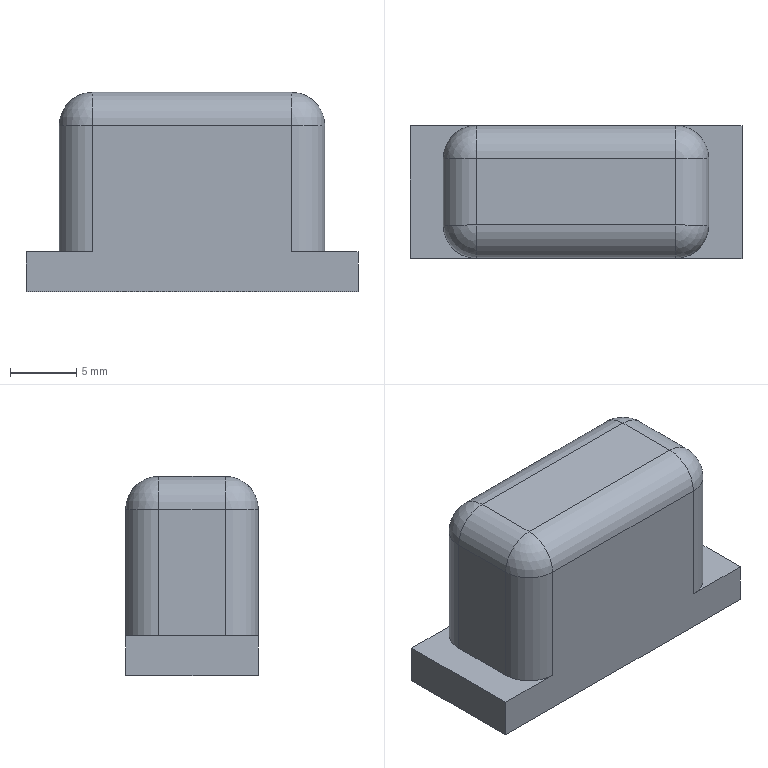Part | NX | 1 solid | 22 faces | box 25 x 10 x 15 mm | volume 3016 mm3 | plane 10 | cylinder 8 | sphere 4 | commonest cylinder face diameters 5 x8
STEP:
#1=CARTESIAN_POINT('',(151.228,185.01,0.));
#2=VERTEX_POINT('',#1);
#3=CARTESIAN_POINT('',(148.728,187.51,0.));
#4=VERTEX_POINT('',#3);
#5=CARTESIAN_POINT('',(148.728,185.01,0.));
#6=DIRECTION('',(0.,0.,1.));
#7=DIRECTION('',(1.,0.,0.));
#8=AXIS2_PLACEMENT_3D('',#5,#6,#7);
#9=CIRCLE('',#8,2.5);
#10=EDGE_CURVE('',#2,#4,#9,.T.);
#11=ORIENTED_EDGE('',*,*,#10,.F.);
#12=CARTESIAN_POINT('',(151.228,180.01,0.));
#13=VERTEX_POINT('',#12);
#14=CARTESIAN_POINT('',(151.228,180.01,0.));
#15=DIRECTION('',(0.,1.,0.));
#16=VECTOR('',#15,1000.);
#17=LINE('',#14,#16);
#18=EDGE_CURVE('',#13,#2,#17,.T.);
#19=ORIENTED_EDGE('',*,*,#18,.F.);
#20=CARTESIAN_POINT('',(148.728,177.51,0.));
#21=VERTEX_POINT('',#20);
#22=CARTESIAN_POINT('',(148.728,180.01,0.));
#23=DIRECTION('',(0.,0.,1.));
#24=DIRECTION('',(1.,0.,0.));
#25=AXIS2_PLACEMENT_3D('',#22,#23,#24);
#26=CIRCLE('',#25,2.5);
#27=EDGE_CURVE('',#21,#13,#26,.T.);
#28=ORIENTED_EDGE('',*,*,#27,.F.);
#29=CARTESIAN_POINT('',(153.728,177.51,0.));
#30=VERTEX_POINT('',#29);
#31=CARTESIAN_POINT('',(153.728,177.51,0.));
#32=DIRECTION('',(-1.,0.,0.));
#33=VECTOR('',#32,1000.);
#34=LINE('',#31,#33);
#35=EDGE_CURVE('',#30,#21,#34,.T.);
#36=ORIENTED_EDGE('',*,*,#35,.F.);
#37=CARTESIAN_POINT('',(153.728,187.51,0.));
#38=VERTEX_POINT('',#37);
#39=CARTESIAN_POINT('',(153.728,187.51,0.));
#40=DIRECTION('',(0.,-1.,0.));
#41=VECTOR('',#40,1000.);
#42=LINE('',#39,#41);
#43=EDGE_CURVE('',#38,#30,#42,.T.);
#44=ORIENTED_EDGE('',*,*,#43,.F.);
#45=CARTESIAN_POINT('',(128.728,187.51,0.));
#46=DIRECTION('',(1.,0.,0.));
#47=VECTOR('',#46,1000.);
#48=LINE('',#45,#47);
#49=EDGE_CURVE('',#4,#38,#48,.T.);
#50=ORIENTED_EDGE('',*,*,#49,.F.);
#51=EDGE_LOOP('',(#11,#19,#28,#36,#44,#50));
#52=FACE_BOUND('',#51,.T.);
#53=CARTESIAN_POINT('',(0.,0.,0.));
#54=DIRECTION('',(0.,0.,-1.));
#55=DIRECTION('',(-1.,0.,0.));
#56=AXIS2_PLACEMENT_3D('',#53,#54,#55);
#57=PLANE('',#56);
#58=ADVANCED_FACE('',(#52),#57,.F.);
#59=CARTESIAN_POINT('',(133.728,187.51,0.));
#60=VERTEX_POINT('',#59);
#61=CARTESIAN_POINT('',(131.228,185.01,0.));
#62=VERTEX_POINT('',#61);
#63=CARTESIAN_POINT('',(133.728,185.01,0.));
#64=DIRECTION('',(0.,0.,1.));
#65=DIRECTION('',(1.,0.,0.));
#66=AXIS2_PLACEMENT_3D('',#63,#64,#65);
#67=CIRCLE('',#66,2.5);
#68=EDGE_CURVE('',#60,#62,#67,.T.);
#69=ORIENTED_EDGE('',*,*,#68,.F.);
#70=CARTESIAN_POINT('',(128.728,187.51,0.));
#71=VERTEX_POINT('',#70);
#72=CARTESIAN_POINT('',(128.728,187.51,0.));
#73=DIRECTION('',(1.,0.,0.));
#74=VECTOR('',#73,1000.);
#75=LINE('',#72,#74);
#76=EDGE_CURVE('',#71,#60,#75,.T.);
#77=ORIENTED_EDGE('',*,*,#76,.F.);
#78=CARTESIAN_POINT('',(128.728,177.51,0.));
#79=VERTEX_POINT('',#78);
#80=CARTESIAN_POINT('',(128.728,177.51,0.));
#81=DIRECTION('',(0.,1.,0.));
#82=VECTOR('',#81,1000.);
#83=LINE('',#80,#82);
#84=EDGE_CURVE('',#79,#71,#83,.T.);
#85=ORIENTED_EDGE('',*,*,#84,.F.);
#86=CARTESIAN_POINT('',(133.728,177.51,0.));
#87=VERTEX_POINT('',#86);
#88=CARTESIAN_POINT('',(153.728,177.51,0.));
#89=DIRECTION('',(-1.,0.,0.));
#90=VECTOR('',#89,1000.);
#91=LINE('',#88,#90);
#92=EDGE_CURVE('',#87,#79,#91,.T.);
#93=ORIENTED_EDGE('',*,*,#92,.F.);
#94=CARTESIAN_POINT('',(131.228,180.01,0.));
#95=VERTEX_POINT('',#94);
#96=CARTESIAN_POINT('',(133.728,180.01,0.));
#97=DIRECTION('',(0.,0.,1.));
#98=DIRECTION('',(1.,0.,0.));
#99=AXIS2_PLACEMENT_3D('',#96,#97,#98);
#100=CIRCLE('',#99,2.5);
#101=EDGE_CURVE('',#95,#87,#100,.T.);
#102=ORIENTED_EDGE('',*,*,#101,.F.);
#103=CARTESIAN_POINT('',(131.228,185.01,0.));
#104=DIRECTION('',(0.,-1.,0.));
#105=VECTOR('',#104,1000.);
#106=LINE('',#103,#105);
#107=EDGE_CURVE('',#62,#95,#106,.T.);
#108=ORIENTED_EDGE('',*,*,#107,.F.);
#109=EDGE_LOOP('',(#69,#77,#85,#93,#102,#108));
#110=FACE_BOUND('',#109,.T.);
#111=CARTESIAN_POINT('',(0.,0.,0.));
#112=DIRECTION('',(0.,0.,-1.));
#113=DIRECTION('',(-1.,0.,0.));
#114=AXIS2_PLACEMENT_3D('',#111,#112,#113);
#115=PLANE('',#114);
#116=ADVANCED_FACE('',(#110),#115,.F.);
#117=CARTESIAN_POINT('',(148.728,177.51,9.5));
#118=VERTEX_POINT('',#117);
#119=CARTESIAN_POINT('',(148.728,177.51,0.));
#120=DIRECTION('',(0.,0.,1.));
#121=VECTOR('',#120,1000.);
#122=LINE('',#119,#121);
#123=EDGE_CURVE('',#21,#118,#122,.T.);
#124=ORIENTED_EDGE('',*,*,#123,.T.);
#125=CARTESIAN_POINT('',(133.728,177.51,9.5));
#126=VERTEX_POINT('',#125);
#127=CARTESIAN_POINT('',(153.728,177.51,9.5));
#128=DIRECTION('',(1.,0.,0.));
#129=VECTOR('',#128,1000.);
#130=LINE('',#127,#129);
#131=EDGE_CURVE('',#118,#126,#130,.F.);
#132=ORIENTED_EDGE('',*,*,#131,.T.);
#133=CARTESIAN_POINT('',(133.728,177.51,0.));
#134=DIRECTION('',(0.,0.,1.));
#135=VECTOR('',#134,1000.);
#136=LINE('',#133,#135);
#137=EDGE_CURVE('',#87,#126,#136,.T.);
#138=ORIENTED_EDGE('',*,*,#137,.F.);
#139=ORIENTED_EDGE('',*,*,#92,.T.);
#140=CARTESIAN_POINT('',(128.728,177.51,-3.));
#141=VERTEX_POINT('',#140);
#142=CARTESIAN_POINT('',(128.728,177.51,0.));
#143=DIRECTION('',(0.,0.,-1.));
#144=VECTOR('',#143,1000.);
#145=LINE('',#142,#144);
#146=EDGE_CURVE('',#79,#141,#145,.T.);
#147=ORIENTED_EDGE('',*,*,#146,.T.);
#148=CARTESIAN_POINT('',(153.728,177.51,-3.));
#149=VERTEX_POINT('',#148);
#150=CARTESIAN_POINT('',(153.728,177.51,-3.));
#151=DIRECTION('',(-1.,0.,0.));
#152=VECTOR('',#151,1000.);
#153=LINE('',#150,#152);
#154=EDGE_CURVE('',#149,#141,#153,.T.);
#155=ORIENTED_EDGE('',*,*,#154,.F.);
#156=CARTESIAN_POINT('',(153.728,177.51,0.));
#157=DIRECTION('',(0.,0.,-1.));
#158=VECTOR('',#157,1000.);
#159=LINE('',#156,#158);
#160=EDGE_CURVE('',#30,#149,#159,.T.);
#161=ORIENTED_EDGE('',*,*,#160,.F.);
#162=ORIENTED_EDGE('',*,*,#35,.T.);
#163=EDGE_LOOP('',(#124,#132,#138,#139,#147,#155,#161,#162));
#164=FACE_BOUND('',#163,.T.);
#165=CARTESIAN_POINT('',(153.728,177.51,0.));
#166=DIRECTION('',(0.,-1.,0.));
#167=DIRECTION('',(0.,0.,-1.));
#168=AXIS2_PLACEMENT_3D('',#165,#166,#167);
#169=PLANE('',#168);
#170=ADVANCED_FACE('',(#164),#169,.T.);
#171=CARTESIAN_POINT('',(128.728,187.51,-3.));
#172=VERTEX_POINT('',#171);
#173=CARTESIAN_POINT('',(128.728,177.51,-3.));
#174=DIRECTION('',(0.,1.,0.));
#175=VECTOR('',#174,1000.);
#176=LINE('',#173,#175);
#177=EDGE_CURVE('',#141,#172,#176,.T.);
#178=ORIENTED_EDGE('',*,*,#177,.F.);
#179=ORIENTED_EDGE('',*,*,#146,.F.);
#180=ORIENTED_EDGE('',*,*,#84,.T.);
#181=CARTESIAN_POINT('',(128.728,187.51,0.));
#182=DIRECTION('',(0.,0.,-1.));
#183=VECTOR('',#182,1000.);
#184=LINE('',#181,#183);
#185=EDGE_CURVE('',#71,#172,#184,.T.);
#186=ORIENTED_EDGE('',*,*,#185,.T.);
#187=EDGE_LOOP('',(#178,#179,#180,#186));
#188=FACE_BOUND('',#187,.T.);
#189=CARTESIAN_POINT('',(128.728,177.51,0.));
#190=DIRECTION('',(-1.,0.,0.));
#191=DIRECTION('',(0.,0.,1.));
#192=AXIS2_PLACEMENT_3D('',#189,#190,#191);
#193=PLANE('',#192);
#194=ADVANCED_FACE('',(#188),#193,.T.);
#195=CARTESIAN_POINT('',(133.728,187.51,9.5));
#196=VERTEX_POINT('',#195);
#197=CARTESIAN_POINT('',(133.728,187.51,0.));
#198=DIRECTION('',(0.,0.,1.));
#199=VECTOR('',#198,1000.);
#200=LINE('',#197,#199);
#201=EDGE_CURVE('',#60,#196,#200,.T.);
#202=ORIENTED_EDGE('',*,*,#201,.T.);
#203=CARTESIAN_POINT('',(148.728,187.51,9.5));
#204=VERTEX_POINT('',#203);
#205=CARTESIAN_POINT('',(128.728,187.51,9.5));
#206=DIRECTION('',(-1.,0.,0.));
#207=VECTOR('',#206,1000.);
#208=LINE('',#205,#207);
#209=EDGE_CURVE('',#196,#204,#208,.F.);
#210=ORIENTED_EDGE('',*,*,#209,.T.);
#211=CARTESIAN_POINT('',(148.728,187.51,0.));
#212=DIRECTION('',(0.,0.,1.));
#213=VECTOR('',#212,1000.);
#214=LINE('',#211,#213);
#215=EDGE_CURVE('',#4,#204,#214,.T.);
#216=ORIENTED_EDGE('',*,*,#215,.F.);
#217=ORIENTED_EDGE('',*,*,#49,.T.);
#218=CARTESIAN_POINT('',(153.728,187.51,-3.));
#219=VERTEX_POINT('',#218);
#220=CARTESIAN_POINT('',(153.728,187.51,0.));
#221=DIRECTION('',(0.,0.,-1.));
#222=VECTOR('',#221,1000.);
#223=LINE('',#220,#222);
#224=EDGE_CURVE('',#38,#219,#223,.T.);
#225=ORIENTED_EDGE('',*,*,#224,.T.);
#226=CARTESIAN_POINT('',(128.728,187.51,-3.));
#227=DIRECTION('',(1.,0.,0.));
#228=VECTOR('',#227,1000.);
#229=LINE('',#226,#228);
#230=EDGE_CURVE('',#172,#219,#229,.T.);
#231=ORIENTED_EDGE('',*,*,#230,.F.);
#232=ORIENTED_EDGE('',*,*,#185,.F.);
#233=ORIENTED_EDGE('',*,*,#76,.T.);
#234=EDGE_LOOP('',(#202,#210,#216,#217,#225,#231,#232,#233));
#235=FACE_BOUND('',#234,.T.);
#236=CARTESIAN_POINT('',(128.728,187.51,0.));
#237=DIRECTION('',(0.,1.,0.));
#238=DIRECTION('',(0.,0.,1.));
#239=AXIS2_PLACEMENT_3D('',#236,#237,#238);
#240=PLANE('',#239);
#241=ADVANCED_FACE('',(#235),#240,.T.);
#242=CARTESIAN_POINT('',(153.728,187.51,-3.));
#243=DIRECTION('',(0.,-1.,0.));
#244=VECTOR('',#243,1000.);
#245=LINE('',#242,#244);
#246=EDGE_CURVE('',#219,#149,#245,.T.);
#247=ORIENTED_EDGE('',*,*,#246,.F.);
#248=ORIENTED_EDGE('',*,*,#224,.F.);
#249=ORIENTED_EDGE('',*,*,#43,.T.);
#250=ORIENTED_EDGE('',*,*,#160,.T.);
#251=EDGE_LOOP('',(#247,#248,#249,#250));
#252=FACE_BOUND('',#251,.T.);
#253=CARTESIAN_POINT('',(153.728,187.51,0.));
#254=DIRECTION('',(1.,0.,0.));
#255=DIRECTION('',(0.,0.,-1.));
#256=AXIS2_PLACEMENT_3D('',#253,#254,#255);
#257=PLANE('',#256);
#258=ADVANCED_FACE('',(#252),#257,.T.);
#259=ORIENTED_EDGE('',*,*,#154,.T.);
#260=ORIENTED_EDGE('',*,*,#177,.T.);
#261=ORIENTED_EDGE('',*,*,#230,.T.);
#262=ORIENTED_EDGE('',*,*,#246,.T.);
#263=EDGE_LOOP('',(#259,#260,#261,#262));
#264=FACE_BOUND('',#263,.T.);
#265=CARTESIAN_POINT('',(0.,0.,-3.));
#266=DIRECTION('',(0.,0.,-1.));
#267=DIRECTION('',(-1.,0.,0.));
#268=AXIS2_PLACEMENT_3D('',#265,#266,#267);
#269=PLANE('',#268);
#270=ADVANCED_FACE('',(#264),#269,.T.);
#271=CARTESIAN_POINT('',(131.228,185.01,9.5));
#272=VERTEX_POINT('',#271);
#273=CARTESIAN_POINT('',(131.228,185.01,0.));
#274=DIRECTION('',(0.,0.,1.));
#275=VECTOR('',#274,1000.);
#276=LINE('',#273,#275);
#277=EDGE_CURVE('',#62,#272,#276,.T.);
#278=ORIENTED_EDGE('',*,*,#277,.T.);
#279=CARTESIAN_POINT('',(133.728,185.01,9.5));
#280=DIRECTION('',(0.,0.,1.));
#281=DIRECTION('',(1.,0.,0.));
#282=AXIS2_PLACEMENT_3D('',#279,#280,#281);
#283=CIRCLE('',#282,2.5);
#284=EDGE_CURVE('',#272,#196,#283,.F.);
#285=ORIENTED_EDGE('',*,*,#284,.T.);
#286=ORIENTED_EDGE('',*,*,#201,.F.);
#287=ORIENTED_EDGE('',*,*,#68,.T.);
#288=EDGE_LOOP('',(#278,#285,#286,#287));
#289=FACE_BOUND('',#288,.T.);
#290=CARTESIAN_POINT('',(133.728,185.01,0.));
#291=DIRECTION('',(0.,0.,1.));
#292=DIRECTION('',(1.,0.,0.));
#293=AXIS2_PLACEMENT_3D('',#290,#291,#292);
#294=CYLINDRICAL_SURFACE('',#293,2.5);
#295=ADVANCED_FACE('',(#289),#294,.T.);
#296=CARTESIAN_POINT('',(131.228,180.01,9.5));
#297=VERTEX_POINT('',#296);
#298=CARTESIAN_POINT('',(131.228,180.01,0.));
#299=DIRECTION('',(0.,0.,1.));
#300=VECTOR('',#299,1000.);
#301=LINE('',#298,#300);
#302=EDGE_CURVE('',#95,#297,#301,.T.);
#303=ORIENTED_EDGE('',*,*,#302,.T.);
#304=CARTESIAN_POINT('',(131.228,185.01,9.5));
#305=DIRECTION('',(0.,-1.,0.));
#306=VECTOR('',#305,1000.);
#307=LINE('',#304,#306);
#308=EDGE_CURVE('',#297,#272,#307,.F.);
#309=ORIENTED_EDGE('',*,*,#308,.T.);
#310=ORIENTED_EDGE('',*,*,#277,.F.);
#311=ORIENTED_EDGE('',*,*,#107,.T.);
#312=EDGE_LOOP('',(#303,#309,#310,#311));
#313=FACE_BOUND('',#312,.T.);
#314=CARTESIAN_POINT('',(131.228,185.01,0.));
#315=DIRECTION('',(-1.,0.,0.));
#316=DIRECTION('',(0.,0.,1.));
#317=AXIS2_PLACEMENT_3D('',#314,#315,#316);
#318=PLANE('',#317);
#319=ADVANCED_FACE('',(#313),#318,.T.);
#320=ORIENTED_EDGE('',*,*,#137,.T.);
#321=CARTESIAN_POINT('',(133.728,180.01,9.5));
#322=DIRECTION('',(0.,0.,1.));
#323=DIRECTION('',(1.,0.,0.));
#324=AXIS2_PLACEMENT_3D('',#321,#322,#323);
#325=CIRCLE('',#324,2.5);
#326=EDGE_CURVE('',#126,#297,#325,.F.);
#327=ORIENTED_EDGE('',*,*,#326,.T.);
#328=ORIENTED_EDGE('',*,*,#302,.F.);
#329=ORIENTED_EDGE('',*,*,#101,.T.);
#330=EDGE_LOOP('',(#320,#327,#328,#329));
#331=FACE_BOUND('',#330,.T.);
#332=CARTESIAN_POINT('',(133.728,180.01,0.));
#333=DIRECTION('',(0.,0.,1.));
#334=DIRECTION('',(1.,0.,0.));
#335=AXIS2_PLACEMENT_3D('',#332,#333,#334);
#336=CYLINDRICAL_SURFACE('',#335,2.5);
#337=ADVANCED_FACE('',(#331),#336,.T.);
#338=CARTESIAN_POINT('',(151.228,180.01,9.5));
#339=VERTEX_POINT('',#338);
#340=CARTESIAN_POINT('',(151.228,180.01,0.));
#341=DIRECTION('',(0.,0.,1.));
#342=VECTOR('',#341,1000.);
#343=LINE('',#340,#342);
#344=EDGE_CURVE('',#13,#339,#343,.T.);
#345=ORIENTED_EDGE('',*,*,#344,.T.);
#346=CARTESIAN_POINT('',(148.728,180.01,9.5));
#347=DIRECTION('',(0.,0.,1.));
#348=DIRECTION('',(1.,0.,0.));
#349=AXIS2_PLACEMENT_3D('',#346,#347,#348);
#350=CIRCLE('',#349,2.5);
#351=EDGE_CURVE('',#339,#118,#350,.F.);
#352=ORIENTED_EDGE('',*,*,#351,.T.);
#353=ORIENTED_EDGE('',*,*,#123,.F.);
#354=ORIENTED_EDGE('',*,*,#27,.T.);
#355=EDGE_LOOP('',(#345,#352,#353,#354));
#356=FACE_BOUND('',#355,.T.);
#357=CARTESIAN_POINT('',(148.728,180.01,0.));
#358=DIRECTION('',(0.,0.,1.));
#359=DIRECTION('',(1.,0.,0.));
#360=AXIS2_PLACEMENT_3D('',#357,#358,#359);
#361=CYLINDRICAL_SURFACE('',#360,2.5);
#362=ADVANCED_FACE('',(#356),#361,.T.);
#363=CARTESIAN_POINT('',(151.228,185.01,9.5));
#364=VERTEX_POINT('',#363);
#365=CARTESIAN_POINT('',(151.228,185.01,0.));
#366=DIRECTION('',(0.,0.,1.));
#367=VECTOR('',#366,1000.);
#368=LINE('',#365,#367);
#369=EDGE_CURVE('',#2,#364,#368,.T.);
#370=ORIENTED_EDGE('',*,*,#369,.T.);
#371=CARTESIAN_POINT('',(151.228,180.01,9.5));
#372=DIRECTION('',(0.,1.,0.));
#373=VECTOR('',#372,1000.);
#374=LINE('',#371,#373);
#375=EDGE_CURVE('',#364,#339,#374,.F.);
#376=ORIENTED_EDGE('',*,*,#375,.T.);
#377=ORIENTED_EDGE('',*,*,#344,.F.);
#378=ORIENTED_EDGE('',*,*,#18,.T.);
#379=EDGE_LOOP('',(#370,#376,#377,#378));
#380=FACE_BOUND('',#379,.T.);
#381=CARTESIAN_POINT('',(151.228,180.01,0.));
#382=DIRECTION('',(1.,0.,0.));
#383=DIRECTION('',(0.,0.,-1.));
#384=AXIS2_PLACEMENT_3D('',#381,#382,#383);
#385=PLANE('',#384);
#386=ADVANCED_FACE('',(#380),#385,.T.);
#387=ORIENTED_EDGE('',*,*,#215,.T.);
#388=CARTESIAN_POINT('',(148.728,185.01,9.5));
#389=DIRECTION('',(0.,0.,1.));
#390=DIRECTION('',(1.,0.,0.));
#391=AXIS2_PLACEMENT_3D('',#388,#389,#390);
#392=CIRCLE('',#391,2.5);
#393=EDGE_CURVE('',#204,#364,#392,.F.);
#394=ORIENTED_EDGE('',*,*,#393,.T.);
#395=ORIENTED_EDGE('',*,*,#369,.F.);
#396=ORIENTED_EDGE('',*,*,#10,.T.);
#397=EDGE_LOOP('',(#387,#394,#395,#396));
#398=FACE_BOUND('',#397,.T.);
#399=CARTESIAN_POINT('',(148.728,185.01,0.));
#400=DIRECTION('',(0.,0.,1.));
#401=DIRECTION('',(1.,0.,0.));
#402=AXIS2_PLACEMENT_3D('',#399,#400,#401);
#403=CYLINDRICAL_SURFACE('',#402,2.5);
#404=ADVANCED_FACE('',(#398),#403,.T.);
#405=CARTESIAN_POINT('',(148.728,185.01,12.));
#406=VERTEX_POINT('',#405);
#407=CARTESIAN_POINT('',(133.728,185.01,12.));
#408=VERTEX_POINT('',#407);
#409=CARTESIAN_POINT('',(133.728,185.01,12.));
#410=DIRECTION('',(-1.,0.,0.));
#411=VECTOR('',#410,1000.);
#412=LINE('',#409,#411);
#413=EDGE_CURVE('',#406,#408,#412,.T.);
#414=ORIENTED_EDGE('',*,*,#413,.T.);
#415=CARTESIAN_POINT('',(133.728,180.01,12.));
#416=VERTEX_POINT('',#415);
#417=CARTESIAN_POINT('',(133.728,185.01,12.));
#418=DIRECTION('',(0.,-1.,0.));
#419=VECTOR('',#418,1000.);
#420=LINE('',#417,#419);
#421=EDGE_CURVE('',#408,#416,#420,.T.);
#422=ORIENTED_EDGE('',*,*,#421,.T.);
#423=CARTESIAN_POINT('',(148.728,180.01,12.));
#424=VERTEX_POINT('',#423);
#425=CARTESIAN_POINT('',(133.728,180.01,12.));
#426=DIRECTION('',(1.,0.,0.));
#427=VECTOR('',#426,1000.);
#428=LINE('',#425,#427);
#429=EDGE_CURVE('',#416,#424,#428,.T.);
#430=ORIENTED_EDGE('',*,*,#429,.T.);
#431=CARTESIAN_POINT('',(148.728,185.01,12.));
#432=DIRECTION('',(0.,1.,0.));
#433=VECTOR('',#432,1000.);
#434=LINE('',#431,#433);
#435=EDGE_CURVE('',#424,#406,#434,.T.);
#436=ORIENTED_EDGE('',*,*,#435,.T.);
#437=EDGE_LOOP('',(#414,#422,#430,#436));
#438=FACE_BOUND('',#437,.T.);
#439=CARTESIAN_POINT('',(133.728,185.01,12.));
#440=DIRECTION('',(0.,0.,1.));
#441=DIRECTION('',(1.,0.,0.));
#442=AXIS2_PLACEMENT_3D('',#439,#440,#441);
#443=PLANE('',#442);
#444=ADVANCED_FACE('',(#438),#443,.T.);
#445=CARTESIAN_POINT('',(148.728,185.01,9.5));
#446=DIRECTION('',(0.,-1.,0.));
#447=DIRECTION('',(0.,0.,-1.));
#448=AXIS2_PLACEMENT_3D('',#445,#446,#447);
#449=CIRCLE('',#448,2.5);
#450=EDGE_CURVE('',#364,#406,#449,.T.);
#451=ORIENTED_EDGE('',*,*,#450,.F.);
#452=ORIENTED_EDGE('',*,*,#393,.F.);
#453=CARTESIAN_POINT('',(148.728,185.01,9.5));
#454=DIRECTION('',(-1.,0.,0.));
#455=DIRECTION('',(0.,0.,1.));
#456=AXIS2_PLACEMENT_3D('',#453,#454,#455);
#457=CIRCLE('',#456,2.5);
#458=EDGE_CURVE('',#406,#204,#457,.T.);
#459=ORIENTED_EDGE('',*,*,#458,.F.);
#460=EDGE_LOOP('',(#451,#452,#459));
#461=FACE_BOUND('',#460,.T.);
#462=CARTESIAN_POINT('',(148.728,185.01,9.5));
#463=DIRECTION('',(0.,0.,1.));
#464=DIRECTION('',(1.,0.,0.));
#465=AXIS2_PLACEMENT_3D('',#462,#463,#464);
#466=SPHERICAL_SURFACE('',#465,2.5);
#467=ADVANCED_FACE('',(#461),#466,.T.);
#468=ORIENTED_EDGE('',*,*,#458,.T.);
#469=ORIENTED_EDGE('',*,*,#209,.F.);
#470=CARTESIAN_POINT('',(133.728,185.01,9.5));
#471=DIRECTION('',(-1.,0.,0.));
#472=DIRECTION('',(0.,0.,1.));
#473=AXIS2_PLACEMENT_3D('',#470,#471,#472);
#474=CIRCLE('',#473,2.5);
#475=EDGE_CURVE('',#408,#196,#474,.T.);
#476=ORIENTED_EDGE('',*,*,#475,.F.);
#477=ORIENTED_EDGE('',*,*,#413,.F.);
#478=EDGE_LOOP('',(#468,#469,#476,#477));
#479=FACE_BOUND('',#478,.T.);
#480=CARTESIAN_POINT('',(133.728,185.01,9.5));
#481=DIRECTION('',(-1.,0.,0.));
#482=DIRECTION('',(0.,0.,1.));
#483=AXIS2_PLACEMENT_3D('',#480,#481,#482);
#484=CYLINDRICAL_SURFACE('',#483,2.5);
#485=ADVANCED_FACE('',(#479),#484,.T.);
#486=ORIENTED_EDGE('',*,*,#450,.T.);
#487=ORIENTED_EDGE('',*,*,#435,.F.);
#488=CARTESIAN_POINT('',(148.728,180.01,9.5));
#489=DIRECTION('',(0.,-1.,0.));
#490=DIRECTION('',(0.,0.,-1.));
#491=AXIS2_PLACEMENT_3D('',#488,#489,#490);
#492=CIRCLE('',#491,2.5);
#493=EDGE_CURVE('',#339,#424,#492,.T.);
#494=ORIENTED_EDGE('',*,*,#493,.F.);
#495=ORIENTED_EDGE('',*,*,#375,.F.);
#496=EDGE_LOOP('',(#486,#487,#494,#495));
#497=FACE_BOUND('',#496,.T.);
#498=CARTESIAN_POINT('',(148.728,185.01,9.5));
#499=DIRECTION('',(0.,1.,0.));
#500=DIRECTION('',(0.,0.,1.));
#501=AXIS2_PLACEMENT_3D('',#498,#499,#500);
#502=CYLINDRICAL_SURFACE('',#501,2.5);
#503=ADVANCED_FACE('',(#497),#502,.T.);
#504=ORIENTED_EDGE('',*,*,#475,.T.);
#505=ORIENTED_EDGE('',*,*,#284,.F.);
#506=CARTESIAN_POINT('',(133.728,185.01,9.5));
#507=DIRECTION('',(0.,-1.,0.));
#508=DIRECTION('',(0.,0.,-1.));
#509=AXIS2_PLACEMENT_3D('',#506,#507,#508);
#510=CIRCLE('',#509,2.5);
#511=EDGE_CURVE('',#408,#272,#510,.T.);
#512=ORIENTED_EDGE('',*,*,#511,.F.);
#513=EDGE_LOOP('',(#504,#505,#512));
#514=FACE_BOUND('',#513,.T.);
#515=CARTESIAN_POINT('',(133.728,185.01,9.5));
#516=DIRECTION('',(0.,0.,1.));
#517=DIRECTION('',(1.,0.,0.));
#518=AXIS2_PLACEMENT_3D('',#515,#516,#517);
#519=SPHERICAL_SURFACE('',#518,2.5);
#520=ADVANCED_FACE('',(#514),#519,.T.);
#521=ORIENTED_EDGE('',*,*,#351,.F.);
#522=ORIENTED_EDGE('',*,*,#493,.T.);
#523=CARTESIAN_POINT('',(148.728,180.01,9.5));
#524=DIRECTION('',(-1.,0.,0.));
#525=DIRECTION('',(0.,-1.,0.));
#526=AXIS2_PLACEMENT_3D('',#523,#524,#525);
#527=CIRCLE('',#526,2.5);
#528=EDGE_CURVE('',#118,#424,#527,.T.);
#529=ORIENTED_EDGE('',*,*,#528,.F.);
#530=EDGE_LOOP('',(#521,#522,#529));
#531=FACE_BOUND('',#530,.T.);
#532=CARTESIAN_POINT('',(148.728,180.01,9.5));
#533=DIRECTION('',(0.,0.,1.));
#534=DIRECTION('',(1.,0.,0.));
#535=AXIS2_PLACEMENT_3D('',#532,#533,#534);
#536=SPHERICAL_SURFACE('',#535,2.5);
#537=ADVANCED_FACE('',(#531),#536,.T.);
#538=ORIENTED_EDGE('',*,*,#511,.T.);
#539=ORIENTED_EDGE('',*,*,#308,.F.);
#540=CARTESIAN_POINT('',(133.728,180.01,9.5));
#541=DIRECTION('',(0.,-1.,0.));
#542=DIRECTION('',(0.,0.,-1.));
#543=AXIS2_PLACEMENT_3D('',#540,#541,#542);
#544=CIRCLE('',#543,2.5);
#545=EDGE_CURVE('',#416,#297,#544,.T.);
#546=ORIENTED_EDGE('',*,*,#545,.F.);
#547=ORIENTED_EDGE('',*,*,#421,.F.);
#548=EDGE_LOOP('',(#538,#539,#546,#547));
#549=FACE_BOUND('',#548,.T.);
#550=CARTESIAN_POINT('',(133.728,185.01,9.5));
#551=DIRECTION('',(0.,-1.,0.));
#552=DIRECTION('',(0.,0.,-1.));
#553=AXIS2_PLACEMENT_3D('',#550,#551,#552);
#554=CYLINDRICAL_SURFACE('',#553,2.5);
#555=ADVANCED_FACE('',(#549),#554,.T.);
#556=ORIENTED_EDGE('',*,*,#528,.T.);
#557=ORIENTED_EDGE('',*,*,#429,.F.);
#558=CARTESIAN_POINT('',(133.728,180.01,9.5));
#559=DIRECTION('',(-1.,0.,0.));
#560=DIRECTION('',(0.,0.,1.));
#561=AXIS2_PLACEMENT_3D('',#558,#559,#560);
#562=CIRCLE('',#561,2.5);
#563=EDGE_CURVE('',#126,#416,#562,.T.);
#564=ORIENTED_EDGE('',*,*,#563,.F.);
#565=ORIENTED_EDGE('',*,*,#131,.F.);
#566=EDGE_LOOP('',(#556,#557,#564,#565));
#567=FACE_BOUND('',#566,.T.);
#568=CARTESIAN_POINT('',(133.728,180.01,9.5));
#569=DIRECTION('',(1.,0.,0.));
#570=DIRECTION('',(0.,0.,-1.));
#571=AXIS2_PLACEMENT_3D('',#568,#569,#570);
#572=CYLINDRICAL_SURFACE('',#571,2.5);
#573=ADVANCED_FACE('',(#567),#572,.T.);
#574=ORIENTED_EDGE('',*,*,#545,.T.);
#575=ORIENTED_EDGE('',*,*,#326,.F.);
#576=ORIENTED_EDGE('',*,*,#563,.T.);
#577=EDGE_LOOP('',(#574,#575,#576));
#578=FACE_BOUND('',#577,.T.);
#579=CARTESIAN_POINT('',(133.728,180.01,9.5));
#580=DIRECTION('',(0.,0.,1.));
#581=DIRECTION('',(1.,0.,0.));
#582=AXIS2_PLACEMENT_3D('',#579,#580,#581);
#583=SPHERICAL_SURFACE('',#582,2.5);
#584=ADVANCED_FACE('',(#578),#583,.T.);
#585=CLOSED_SHELL('',(#58,#116,#170,#194,#241,#258,#270,#295,#319,#337,#362,#386,#404,#444,#467,#485,#503,#520,#537,#555,#573,#584));
#586=MANIFOLD_SOLID_BREP('',#585);
#587=(LENGTH_UNIT()NAMED_UNIT(*)SI_UNIT(.MILLI.,.METRE.));
#588=UNCERTAINTY_MEASURE_WITH_UNIT(LENGTH_MEASURE(0.00001),#587,'','');
#589=(NAMED_UNIT(*)PLANE_ANGLE_UNIT()SI_UNIT($,.RADIAN.));
#590=(NAMED_UNIT(*)SI_UNIT($,.STERADIAN.)SOLID_ANGLE_UNIT());
#591=(GEOMETRIC_REPRESENTATION_CONTEXT(3)GLOBAL_UNCERTAINTY_ASSIGNED_CONTEXT((#588))GLOBAL_UNIT_ASSIGNED_CONTEXT((#587,#589,#590))REPRESENTATION_CONTEXT('',''));
#592=ADVANCED_BREP_SHAPE_REPRESENTATION('',(#586),#591);